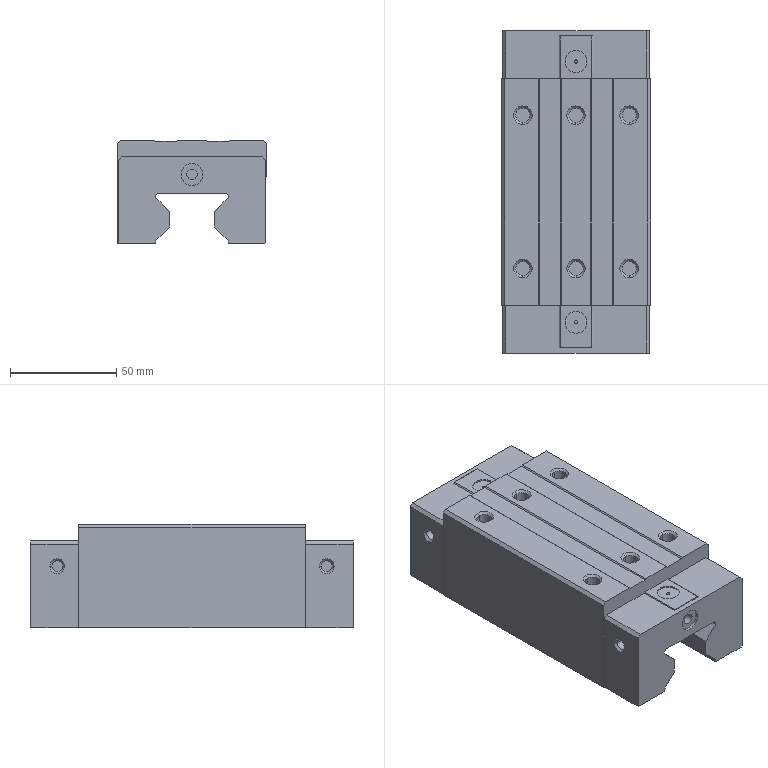Part | STEP file | Chamfer 6-2 | 1 solid | 127 faces | box 70 x 151.5 x 48.5 mm | volume 387340 mm3 | plane 71 | cylinder 36 | cone 20 | commonest cylinder face diameters 5 x12 6.75 x12 10.3 x8 1.5 x4